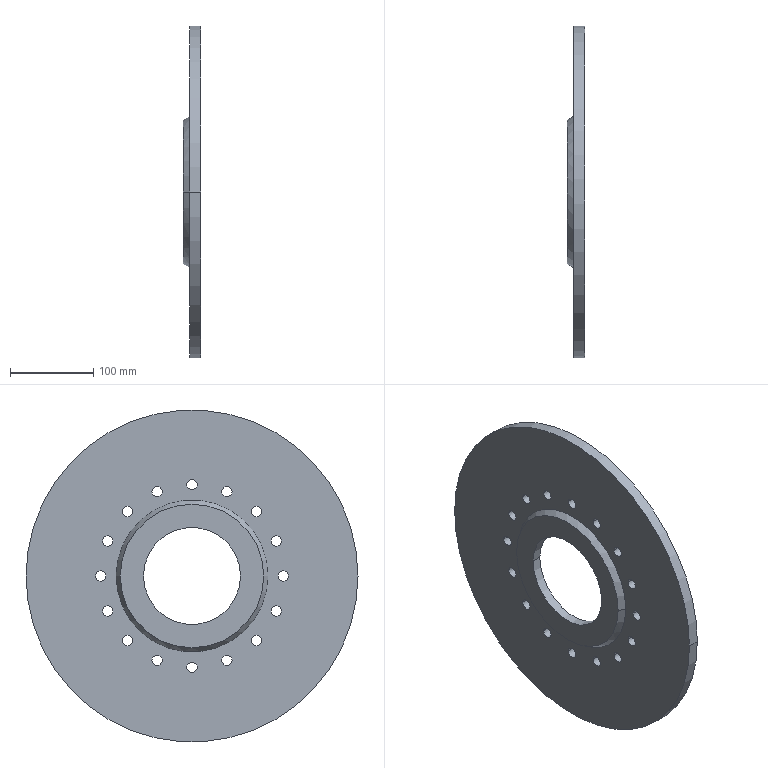Part | NX | features BREP 1 | 1 solid | 44 faces | box 21.5 x 400 x 400 mm | volume 1510380 mm3 | cylinder 38 | plane 4 | cone 2 | commonest cylinder face diameters 12.5 x32 117 x2 173 x2 400 x2
STEP:
#1=CARTESIAN_POINT('',(-403.355,-86.5,0.));
#2=VERTEX_POINT('',#1);
#3=CARTESIAN_POINT('',(-395.355,-91.5,0.));
#4=VERTEX_POINT('',#3);
#5=CARTESIAN_POINT('',(-403.355,-86.5,0.));
#6=DIRECTION('',(0.848,-0.53,0.));
#7=VECTOR('',#6,1000.);
#8=LINE('',#5,#7);
#9=EDGE_CURVE('',#2,#4,#8,.T.);
#10=ORIENTED_EDGE('',*,*,#9,.T.);
#11=CARTESIAN_POINT('',(-395.355,91.5,0.));
#12=VERTEX_POINT('',#11);
#13=CARTESIAN_POINT('',(-395.355,0.,0.));
#14=DIRECTION('',(-1.,0.,0.));
#15=DIRECTION('',(0.,-1.,0.));
#16=AXIS2_PLACEMENT_3D('',#13,#14,#15);
#17=CIRCLE('',#16,91.5);
#18=EDGE_CURVE('',#4,#12,#17,.T.);
#19=ORIENTED_EDGE('',*,*,#18,.T.);
#20=CARTESIAN_POINT('',(-403.355,86.5,0.));
#21=VERTEX_POINT('',#20);
#22=CARTESIAN_POINT('',(-403.355,86.5,0.));
#23=DIRECTION('',(0.848,0.53,0.));
#24=VECTOR('',#23,1000.);
#25=LINE('',#22,#24);
#26=EDGE_CURVE('',#21,#12,#25,.T.);
#27=ORIENTED_EDGE('',*,*,#26,.F.);
#28=CARTESIAN_POINT('',(-403.355,0.,0.));
#29=DIRECTION('',(-1.,0.,0.));
#30=DIRECTION('',(0.,-1.,0.));
#31=AXIS2_PLACEMENT_3D('',#28,#29,#30);
#32=CIRCLE('',#31,86.5);
#33=EDGE_CURVE('',#2,#21,#32,.T.);
#34=ORIENTED_EDGE('',*,*,#33,.F.);
#35=EDGE_LOOP('',(#10,#19,#27,#34));
#36=FACE_BOUND('',#35,.T.);
#37=CARTESIAN_POINT('',(-403.355,0.,0.));
#38=DIRECTION('',(1.,0.,0.));
#39=DIRECTION('',(0.,-1.,0.));
#40=AXIS2_PLACEMENT_3D('',#37,#38,#39);
#41=CONICAL_SURFACE('',#40,86.5,0.5586);
#42=ADVANCED_FACE('',(#36),#41,.T.);
#43=CARTESIAN_POINT('',(-395.355,107.877,42.095));
#44=VERTEX_POINT('',#43);
#45=CARTESIAN_POINT('',(-381.855,107.877,42.095));
#46=VERTEX_POINT('',#45);
#47=CARTESIAN_POINT('',(-381.855,107.877,42.095));
#48=DIRECTION('',(-1.,0.,0.));
#49=VECTOR('',#48,1000.);
#50=LINE('',#47,#49);
#51=EDGE_CURVE('',#44,#46,#50,.F.);
#52=ORIENTED_EDGE('',*,*,#51,.F.);
#53=CARTESIAN_POINT('',(-395.355,95.377,42.095));
#54=VERTEX_POINT('',#53);
#55=CARTESIAN_POINT('',(-395.355,101.627,42.095));
#56=DIRECTION('',(-1.,0.,0.));
#57=DIRECTION('',(0.,-1.,0.));
#58=AXIS2_PLACEMENT_3D('',#55,#56,#57);
#59=CIRCLE('',#58,6.25);
#60=EDGE_CURVE('',#44,#54,#59,.T.);
#61=ORIENTED_EDGE('',*,*,#60,.T.);
#62=CARTESIAN_POINT('',(-381.855,95.377,42.095));
#63=VERTEX_POINT('',#62);
#64=CARTESIAN_POINT('',(-381.855,95.377,42.095));
#65=DIRECTION('',(-1.,0.,0.));
#66=VECTOR('',#65,1000.);
#67=LINE('',#64,#66);
#68=EDGE_CURVE('',#54,#63,#67,.F.);
#69=ORIENTED_EDGE('',*,*,#68,.T.);
#70=CARTESIAN_POINT('',(-381.855,101.627,42.095));
#71=DIRECTION('',(-1.,0.,0.));
#72=DIRECTION('',(0.,-1.,0.));
#73=AXIS2_PLACEMENT_3D('',#70,#71,#72);
#74=CIRCLE('',#73,6.25);
#75=EDGE_CURVE('',#46,#63,#74,.T.);
#76=ORIENTED_EDGE('',*,*,#75,.F.);
#77=EDGE_LOOP('',(#52,#61,#69,#76));
#78=FACE_BOUND('',#77,.T.);
#79=CARTESIAN_POINT('',(-381.855,101.627,42.095));
#80=DIRECTION('',(-1.,0.,0.));
#81=DIRECTION('',(0.,1.,0.));
#82=AXIS2_PLACEMENT_3D('',#79,#80,#81);
#83=CYLINDRICAL_SURFACE('',#82,6.25);
#84=ADVANCED_FACE('',(#78),#83,.F.);
#85=CARTESIAN_POINT('',(-395.355,84.032,77.782));
#86=VERTEX_POINT('',#85);
#87=CARTESIAN_POINT('',(-381.855,84.032,77.782));
#88=VERTEX_POINT('',#87);
#89=CARTESIAN_POINT('',(-381.855,84.032,77.782));
#90=DIRECTION('',(-1.,0.,0.));
#91=VECTOR('',#90,1000.);
#92=LINE('',#89,#91);
#93=EDGE_CURVE('',#86,#88,#92,.F.);
#94=ORIENTED_EDGE('',*,*,#93,.F.);
#95=CARTESIAN_POINT('',(-395.355,71.532,77.782));
#96=VERTEX_POINT('',#95);
#97=CARTESIAN_POINT('',(-395.355,77.782,77.782));
#98=DIRECTION('',(-1.,0.,0.));
#99=DIRECTION('',(0.,-1.,0.));
#100=AXIS2_PLACEMENT_3D('',#97,#98,#99);
#101=CIRCLE('',#100,6.25);
#102=EDGE_CURVE('',#86,#96,#101,.T.);
#103=ORIENTED_EDGE('',*,*,#102,.T.);
#104=CARTESIAN_POINT('',(-381.855,71.532,77.782));
#105=VERTEX_POINT('',#104);
#106=CARTESIAN_POINT('',(-381.855,71.532,77.782));
#107=DIRECTION('',(-1.,0.,0.));
#108=VECTOR('',#107,1000.);
#109=LINE('',#106,#108);
#110=EDGE_CURVE('',#96,#105,#109,.F.);
#111=ORIENTED_EDGE('',*,*,#110,.T.);
#112=CARTESIAN_POINT('',(-381.855,77.782,77.782));
#113=DIRECTION('',(-1.,0.,0.));
#114=DIRECTION('',(0.,-1.,0.));
#115=AXIS2_PLACEMENT_3D('',#112,#113,#114);
#116=CIRCLE('',#115,6.25);
#117=EDGE_CURVE('',#88,#105,#116,.T.);
#118=ORIENTED_EDGE('',*,*,#117,.F.);
#119=EDGE_LOOP('',(#94,#103,#111,#118));
#120=FACE_BOUND('',#119,.T.);
#121=CARTESIAN_POINT('',(-381.855,77.782,77.782));
#122=DIRECTION('',(-1.,0.,0.));
#123=DIRECTION('',(0.,1.,0.));
#124=AXIS2_PLACEMENT_3D('',#121,#122,#123);
#125=CYLINDRICAL_SURFACE('',#124,6.25);
#126=ADVANCED_FACE('',(#120),#125,.F.);
#127=CARTESIAN_POINT('',(-395.355,48.345,101.627));
#128=VERTEX_POINT('',#127);
#129=CARTESIAN_POINT('',(-381.855,48.345,101.627));
#130=VERTEX_POINT('',#129);
#131=CARTESIAN_POINT('',(-381.855,48.345,101.627));
#132=DIRECTION('',(-1.,0.,0.));
#133=VECTOR('',#132,1000.);
#134=LINE('',#131,#133);
#135=EDGE_CURVE('',#128,#130,#134,.F.);
#136=ORIENTED_EDGE('',*,*,#135,.F.);
#137=CARTESIAN_POINT('',(-395.355,35.845,101.627));
#138=VERTEX_POINT('',#137);
#139=CARTESIAN_POINT('',(-395.355,42.095,101.627));
#140=DIRECTION('',(-1.,0.,0.));
#141=DIRECTION('',(0.,-1.,0.));
#142=AXIS2_PLACEMENT_3D('',#139,#140,#141);
#143=CIRCLE('',#142,6.25);
#144=EDGE_CURVE('',#128,#138,#143,.T.);
#145=ORIENTED_EDGE('',*,*,#144,.T.);
#146=CARTESIAN_POINT('',(-381.855,35.845,101.627));
#147=VERTEX_POINT('',#146);
#148=CARTESIAN_POINT('',(-381.855,35.845,101.627));
#149=DIRECTION('',(-1.,0.,0.));
#150=VECTOR('',#149,1000.);
#151=LINE('',#148,#150);
#152=EDGE_CURVE('',#138,#147,#151,.F.);
#153=ORIENTED_EDGE('',*,*,#152,.T.);
#154=CARTESIAN_POINT('',(-381.855,42.095,101.627));
#155=DIRECTION('',(-1.,0.,0.));
#156=DIRECTION('',(0.,-1.,0.));
#157=AXIS2_PLACEMENT_3D('',#154,#155,#156);
#158=CIRCLE('',#157,6.25);
#159=EDGE_CURVE('',#130,#147,#158,.T.);
#160=ORIENTED_EDGE('',*,*,#159,.F.);
#161=EDGE_LOOP('',(#136,#145,#153,#160));
#162=FACE_BOUND('',#161,.T.);
#163=CARTESIAN_POINT('',(-381.855,42.095,101.627));
#164=DIRECTION('',(-1.,0.,0.));
#165=DIRECTION('',(0.,1.,0.));
#166=AXIS2_PLACEMENT_3D('',#163,#164,#165);
#167=CYLINDRICAL_SURFACE('',#166,6.25);
#168=ADVANCED_FACE('',(#162),#167,.F.);
#169=CARTESIAN_POINT('',(-395.355,6.25,110.));
#170=VERTEX_POINT('',#169);
#171=CARTESIAN_POINT('',(-381.855,6.25,110.));
#172=VERTEX_POINT('',#171);
#173=CARTESIAN_POINT('',(-381.855,6.25,110.));
#174=DIRECTION('',(-1.,0.,0.));
#175=VECTOR('',#174,1000.);
#176=LINE('',#173,#175);
#177=EDGE_CURVE('',#170,#172,#176,.F.);
#178=ORIENTED_EDGE('',*,*,#177,.F.);
#179=CARTESIAN_POINT('',(-395.355,-6.25,110.));
#180=VERTEX_POINT('',#179);
#181=CARTESIAN_POINT('',(-395.355,0.,110.));
#182=DIRECTION('',(-1.,0.,0.));
#183=DIRECTION('',(0.,-1.,0.));
#184=AXIS2_PLACEMENT_3D('',#181,#182,#183);
#185=CIRCLE('',#184,6.25);
#186=EDGE_CURVE('',#170,#180,#185,.T.);
#187=ORIENTED_EDGE('',*,*,#186,.T.);
#188=CARTESIAN_POINT('',(-381.855,-6.25,110.));
#189=VERTEX_POINT('',#188);
#190=CARTESIAN_POINT('',(-381.855,-6.25,110.));
#191=DIRECTION('',(-1.,0.,0.));
#192=VECTOR('',#191,1000.);
#193=LINE('',#190,#192);
#194=EDGE_CURVE('',#180,#189,#193,.F.);
#195=ORIENTED_EDGE('',*,*,#194,.T.);
#196=CARTESIAN_POINT('',(-381.855,0.,110.));
#197=DIRECTION('',(-1.,0.,0.));
#198=DIRECTION('',(0.,-1.,0.));
#199=AXIS2_PLACEMENT_3D('',#196,#197,#198);
#200=CIRCLE('',#199,6.25);
#201=EDGE_CURVE('',#172,#189,#200,.T.);
#202=ORIENTED_EDGE('',*,*,#201,.F.);
#203=EDGE_LOOP('',(#178,#187,#195,#202));
#204=FACE_BOUND('',#203,.T.);
#205=CARTESIAN_POINT('',(-381.855,0.,110.));
#206=DIRECTION('',(-1.,0.,0.));
#207=DIRECTION('',(0.,1.,0.));
#208=AXIS2_PLACEMENT_3D('',#205,#206,#207);
#209=CYLINDRICAL_SURFACE('',#208,6.25);
#210=ADVANCED_FACE('',(#204),#209,.F.);
#211=CARTESIAN_POINT('',(-395.355,-35.845,101.627));
#212=VERTEX_POINT('',#211);
#213=CARTESIAN_POINT('',(-381.855,-35.845,101.627));
#214=VERTEX_POINT('',#213);
#215=CARTESIAN_POINT('',(-381.855,-35.845,101.627));
#216=DIRECTION('',(-1.,0.,0.));
#217=VECTOR('',#216,1000.);
#218=LINE('',#215,#217);
#219=EDGE_CURVE('',#212,#214,#218,.F.);
#220=ORIENTED_EDGE('',*,*,#219,.F.);
#221=CARTESIAN_POINT('',(-395.355,-48.345,101.627));
#222=VERTEX_POINT('',#221);
#223=CARTESIAN_POINT('',(-395.355,-42.095,101.627));
#224=DIRECTION('',(-1.,0.,0.));
#225=DIRECTION('',(0.,-1.,0.));
#226=AXIS2_PLACEMENT_3D('',#223,#224,#225);
#227=CIRCLE('',#226,6.25);
#228=EDGE_CURVE('',#212,#222,#227,.T.);
#229=ORIENTED_EDGE('',*,*,#228,.T.);
#230=CARTESIAN_POINT('',(-381.855,-48.345,101.627));
#231=VERTEX_POINT('',#230);
#232=CARTESIAN_POINT('',(-381.855,-48.345,101.627));
#233=DIRECTION('',(-1.,0.,0.));
#234=VECTOR('',#233,1000.);
#235=LINE('',#232,#234);
#236=EDGE_CURVE('',#222,#231,#235,.F.);
#237=ORIENTED_EDGE('',*,*,#236,.T.);
#238=CARTESIAN_POINT('',(-381.855,-42.095,101.627));
#239=DIRECTION('',(-1.,0.,0.));
#240=DIRECTION('',(0.,-1.,0.));
#241=AXIS2_PLACEMENT_3D('',#238,#239,#240);
#242=CIRCLE('',#241,6.25);
#243=EDGE_CURVE('',#214,#231,#242,.T.);
#244=ORIENTED_EDGE('',*,*,#243,.F.);
#245=EDGE_LOOP('',(#220,#229,#237,#244));
#246=FACE_BOUND('',#245,.T.);
#247=CARTESIAN_POINT('',(-381.855,-42.095,101.627));
#248=DIRECTION('',(-1.,0.,0.));
#249=DIRECTION('',(0.,1.,0.));
#250=AXIS2_PLACEMENT_3D('',#247,#248,#249);
#251=CYLINDRICAL_SURFACE('',#250,6.25);
#252=ADVANCED_FACE('',(#246),#251,.F.);
#253=CARTESIAN_POINT('',(-395.355,-71.532,77.782));
#254=VERTEX_POINT('',#253);
#255=CARTESIAN_POINT('',(-381.855,-71.532,77.782));
#256=VERTEX_POINT('',#255);
#257=CARTESIAN_POINT('',(-381.855,-71.532,77.782));
#258=DIRECTION('',(-1.,0.,0.));
#259=VECTOR('',#258,1000.);
#260=LINE('',#257,#259);
#261=EDGE_CURVE('',#254,#256,#260,.F.);
#262=ORIENTED_EDGE('',*,*,#261,.F.);
#263=CARTESIAN_POINT('',(-395.355,-84.032,77.782));
#264=VERTEX_POINT('',#263);
#265=CARTESIAN_POINT('',(-395.355,-77.782,77.782));
#266=DIRECTION('',(-1.,0.,0.));
#267=DIRECTION('',(0.,-1.,0.));
#268=AXIS2_PLACEMENT_3D('',#265,#266,#267);
#269=CIRCLE('',#268,6.25);
#270=EDGE_CURVE('',#254,#264,#269,.T.);
#271=ORIENTED_EDGE('',*,*,#270,.T.);
#272=CARTESIAN_POINT('',(-381.855,-84.032,77.782));
#273=VERTEX_POINT('',#272);
#274=CARTESIAN_POINT('',(-381.855,-84.032,77.782));
#275=DIRECTION('',(-1.,0.,0.));
#276=VECTOR('',#275,1000.);
#277=LINE('',#274,#276);
#278=EDGE_CURVE('',#264,#273,#277,.F.);
#279=ORIENTED_EDGE('',*,*,#278,.T.);
#280=CARTESIAN_POINT('',(-381.855,-77.782,77.782));
#281=DIRECTION('',(-1.,0.,0.));
#282=DIRECTION('',(0.,-1.,0.));
#283=AXIS2_PLACEMENT_3D('',#280,#281,#282);
#284=CIRCLE('',#283,6.25);
#285=EDGE_CURVE('',#256,#273,#284,.T.);
#286=ORIENTED_EDGE('',*,*,#285,.F.);
#287=EDGE_LOOP('',(#262,#271,#279,#286));
#288=FACE_BOUND('',#287,.T.);
#289=CARTESIAN_POINT('',(-381.855,-77.782,77.782));
#290=DIRECTION('',(-1.,0.,0.));
#291=DIRECTION('',(0.,1.,0.));
#292=AXIS2_PLACEMENT_3D('',#289,#290,#291);
#293=CYLINDRICAL_SURFACE('',#292,6.25);
#294=ADVANCED_FACE('',(#288),#293,.F.);
#295=CARTESIAN_POINT('',(-395.355,-95.377,42.095));
#296=VERTEX_POINT('',#295);
#297=CARTESIAN_POINT('',(-381.855,-95.377,42.095));
#298=VERTEX_POINT('',#297);
#299=CARTESIAN_POINT('',(-381.855,-95.377,42.095));
#300=DIRECTION('',(-1.,0.,0.));
#301=VECTOR('',#300,1000.);
#302=LINE('',#299,#301);
#303=EDGE_CURVE('',#296,#298,#302,.F.);
#304=ORIENTED_EDGE('',*,*,#303,.F.);
#305=CARTESIAN_POINT('',(-395.355,-107.877,42.095));
#306=VERTEX_POINT('',#305);
#307=CARTESIAN_POINT('',(-395.355,-101.627,42.095));
#308=DIRECTION('',(-1.,0.,0.));
#309=DIRECTION('',(0.,-1.,0.));
#310=AXIS2_PLACEMENT_3D('',#307,#308,#309);
#311=CIRCLE('',#310,6.25);
#312=EDGE_CURVE('',#296,#306,#311,.T.);
#313=ORIENTED_EDGE('',*,*,#312,.T.);
#314=CARTESIAN_POINT('',(-381.855,-107.877,42.095));
#315=VERTEX_POINT('',#314);
#316=CARTESIAN_POINT('',(-381.855,-107.877,42.095));
#317=DIRECTION('',(-1.,0.,0.));
#318=VECTOR('',#317,1000.);
#319=LINE('',#316,#318);
#320=EDGE_CURVE('',#306,#315,#319,.F.);
#321=ORIENTED_EDGE('',*,*,#320,.T.);
#322=CARTESIAN_POINT('',(-381.855,-101.627,42.095));
#323=DIRECTION('',(-1.,0.,0.));
#324=DIRECTION('',(0.,-1.,0.));
#325=AXIS2_PLACEMENT_3D('',#322,#323,#324);
#326=CIRCLE('',#325,6.25);
#327=EDGE_CURVE('',#298,#315,#326,.T.);
#328=ORIENTED_EDGE('',*,*,#327,.F.);
#329=EDGE_LOOP('',(#304,#313,#321,#328));
#330=FACE_BOUND('',#329,.T.);
#331=CARTESIAN_POINT('',(-381.855,-101.627,42.095));
#332=DIRECTION('',(-1.,0.,0.));
#333=DIRECTION('',(0.,1.,0.));
#334=AXIS2_PLACEMENT_3D('',#331,#332,#333);
#335=CYLINDRICAL_SURFACE('',#334,6.25);
#336=ADVANCED_FACE('',(#330),#335,.F.);
#337=CARTESIAN_POINT('',(-395.355,-103.75,0.));
#338=VERTEX_POINT('',#337);
#339=CARTESIAN_POINT('',(-381.855,-103.75,0.));
#340=VERTEX_POINT('',#339);
#341=CARTESIAN_POINT('',(-381.855,-103.75,0.));
#342=DIRECTION('',(-1.,0.,0.));
#343=VECTOR('',#342,1000.);
#344=LINE('',#341,#343);
#345=EDGE_CURVE('',#338,#340,#344,.F.);
#346=ORIENTED_EDGE('',*,*,#345,.F.);
#347=CARTESIAN_POINT('',(-395.355,-116.25,0.));
#348=VERTEX_POINT('',#347);
#349=CARTESIAN_POINT('',(-395.355,-110.,0.));
#350=DIRECTION('',(-1.,0.,0.));
#351=DIRECTION('',(0.,-1.,0.));
#352=AXIS2_PLACEMENT_3D('',#349,#350,#351);
#353=CIRCLE('',#352,6.25);
#354=EDGE_CURVE('',#338,#348,#353,.T.);
#355=ORIENTED_EDGE('',*,*,#354,.T.);
#356=CARTESIAN_POINT('',(-381.855,-116.25,0.));
#357=VERTEX_POINT('',#356);
#358=CARTESIAN_POINT('',(-381.855,-116.25,0.));
#359=DIRECTION('',(-1.,0.,0.));
#360=VECTOR('',#359,1000.);
#361=LINE('',#358,#360);
#362=EDGE_CURVE('',#348,#357,#361,.F.);
#363=ORIENTED_EDGE('',*,*,#362,.T.);
#364=CARTESIAN_POINT('',(-381.855,-110.,0.));
#365=DIRECTION('',(-1.,0.,0.));
#366=DIRECTION('',(0.,-1.,0.));
#367=AXIS2_PLACEMENT_3D('',#364,#365,#366);
#368=CIRCLE('',#367,6.25);
#369=EDGE_CURVE('',#340,#357,#368,.T.);
#370=ORIENTED_EDGE('',*,*,#369,.F.);
#371=EDGE_LOOP('',(#346,#355,#363,#370));
#372=FACE_BOUND('',#371,.T.);
#373=CARTESIAN_POINT('',(-381.855,-110.,0.));
#374=DIRECTION('',(-1.,0.,0.));
#375=DIRECTION('',(0.,1.,0.));
#376=AXIS2_PLACEMENT_3D('',#373,#374,#375);
#377=CYLINDRICAL_SURFACE('',#376,6.25);
#378=ADVANCED_FACE('',(#372),#377,.F.);
#379=CARTESIAN_POINT('',(-395.355,-95.377,-42.095));
#380=VERTEX_POINT('',#379);
#381=CARTESIAN_POINT('',(-381.855,-95.377,-42.095));
#382=VERTEX_POINT('',#381);
#383=CARTESIAN_POINT('',(-381.855,-95.377,-42.095));
#384=DIRECTION('',(-1.,0.,0.));
#385=VECTOR('',#384,1000.);
#386=LINE('',#383,#385);
#387=EDGE_CURVE('',#380,#382,#386,.F.);
#388=ORIENTED_EDGE('',*,*,#387,.F.);
#389=CARTESIAN_POINT('',(-395.355,-107.877,-42.095));
#390=VERTEX_POINT('',#389);
#391=CARTESIAN_POINT('',(-395.355,-101.627,-42.095));
#392=DIRECTION('',(-1.,0.,0.));
#393=DIRECTION('',(0.,-1.,0.));
#394=AXIS2_PLACEMENT_3D('',#391,#392,#393);
#395=CIRCLE('',#394,6.25);
#396=EDGE_CURVE('',#380,#390,#395,.T.);
#397=ORIENTED_EDGE('',*,*,#396,.T.);
#398=CARTESIAN_POINT('',(-381.855,-107.877,-42.095));
#399=VERTEX_POINT('',#398);
#400=CARTESIAN_POINT('',(-381.855,-107.877,-42.095));
#401=DIRECTION('',(-1.,0.,0.));
#402=VECTOR('',#401,1000.);
#403=LINE('',#400,#402);
#404=EDGE_CURVE('',#390,#399,#403,.F.);
#405=ORIENTED_EDGE('',*,*,#404,.T.);
#406=CARTESIAN_POINT('',(-381.855,-101.627,-42.095));
#407=DIRECTION('',(-1.,0.,0.));
#408=DIRECTION('',(0.,-1.,0.));
#409=AXIS2_PLACEMENT_3D('',#406,#407,#408);
#410=CIRCLE('',#409,6.25);
#411=EDGE_CURVE('',#382,#399,#410,.T.);
#412=ORIENTED_EDGE('',*,*,#411,.F.);
#413=EDGE_LOOP('',(#388,#397,#405,#412));
#414=FACE_BOUND('',#413,.T.);
#415=CARTESIAN_POINT('',(-381.855,-101.627,-42.095));
#416=DIRECTION('',(-1.,0.,0.));
#417=DIRECTION('',(0.,1.,0.));
#418=AXIS2_PLACEMENT_3D('',#415,#416,#417);
#419=CYLINDRICAL_SURFACE('',#418,6.25);
#420=ADVANCED_FACE('',(#414),#419,.F.);
#421=CARTESIAN_POINT('',(-395.355,-71.532,-77.782));
#422=VERTEX_POINT('',#421);
#423=CARTESIAN_POINT('',(-381.855,-71.532,-77.782));
#424=VERTEX_POINT('',#423);
#425=CARTESIAN_POINT('',(-381.855,-71.532,-77.782));
#426=DIRECTION('',(-1.,0.,0.));
#427=VECTOR('',#426,1000.);
#428=LINE('',#425,#427);
#429=EDGE_CURVE('',#422,#424,#428,.F.);
#430=ORIENTED_EDGE('',*,*,#429,.F.);
#431=CARTESIAN_POINT('',(-395.355,-84.032,-77.782));
#432=VERTEX_POINT('',#431);
#433=CARTESIAN_POINT('',(-395.355,-77.782,-77.782));
#434=DIRECTION('',(-1.,0.,0.));
#435=DIRECTION('',(0.,-1.,0.));
#436=AXIS2_PLACEMENT_3D('',#433,#434,#435);
#437=CIRCLE('',#436,6.25);
#438=EDGE_CURVE('',#422,#432,#437,.T.);
#439=ORIENTED_EDGE('',*,*,#438,.T.);
#440=CARTESIAN_POINT('',(-381.855,-84.032,-77.782));
#441=VERTEX_POINT('',#440);
#442=CARTESIAN_POINT('',(-381.855,-84.032,-77.782));
#443=DIRECTION('',(-1.,0.,0.));
#444=VECTOR('',#443,1000.);
#445=LINE('',#442,#444);
#446=EDGE_CURVE('',#432,#441,#445,.F.);
#447=ORIENTED_EDGE('',*,*,#446,.T.);
#448=CARTESIAN_POINT('',(-381.855,-77.782,-77.782));
#449=DIRECTION('',(-1.,0.,0.));
#450=DIRECTION('',(0.,-1.,0.));
#451=AXIS2_PLACEMENT_3D('',#448,#449,#450);
#452=CIRCLE('',#451,6.25);
#453=EDGE_CURVE('',#424,#441,#452,.T.);
#454=ORIENTED_EDGE('',*,*,#453,.F.);
#455=EDGE_LOOP('',(#430,#439,#447,#454));
#456=FACE_BOUND('',#455,.T.);
#457=CARTESIAN_POINT('',(-381.855,-77.782,-77.782));
#458=DIRECTION('',(-1.,0.,0.));
#459=DIRECTION('',(0.,1.,0.));
#460=AXIS2_PLACEMENT_3D('',#457,#458,#459);
#461=CYLINDRICAL_SURFACE('',#460,6.25);
#462=ADVANCED_FACE('',(#456),#461,.F.);
#463=CARTESIAN_POINT('',(-395.355,-35.845,-101.627));
#464=VERTEX_POINT('',#463);
#465=CARTESIAN_POINT('',(-381.855,-35.845,-101.627));
#466=VERTEX_POINT('',#465);
#467=CARTESIAN_POINT('',(-381.855,-35.845,-101.627));
#468=DIRECTION('',(-1.,0.,0.));
#469=VECTOR('',#468,1000.);
#470=LINE('',#467,#469);
#471=EDGE_CURVE('',#464,#466,#470,.F.);
#472=ORIENTED_EDGE('',*,*,#471,.F.);
#473=CARTESIAN_POINT('',(-395.355,-48.345,-101.627));
#474=VERTEX_POINT('',#473);
#475=CARTESIAN_POINT('',(-395.355,-42.095,-101.627));
#476=DIRECTION('',(-1.,0.,0.));
#477=DIRECTION('',(0.,-1.,0.));
#478=AXIS2_PLACEMENT_3D('',#475,#476,#477);
#479=CIRCLE('',#478,6.25);
#480=EDGE_CURVE('',#464,#474,#479,.T.);
#481=ORIENTED_EDGE('',*,*,#480,.T.);
#482=CARTESIAN_POINT('',(-381.855,-48.345,-101.627));
#483=VERTEX_POINT('',#482);
#484=CARTESIAN_POINT('',(-381.855,-48.345,-101.627));
#485=DIRECTION('',(-1.,0.,0.));
#486=VECTOR('',#485,1000.);
#487=LINE('',#484,#486);
#488=EDGE_CURVE('',#474,#483,#487,.F.);
#489=ORIENTED_EDGE('',*,*,#488,.T.);
#490=CARTESIAN_POINT('',(-381.855,-42.095,-101.627));
#491=DIRECTION('',(-1.,0.,0.));
#492=DIRECTION('',(0.,-1.,0.));
#493=AXIS2_PLACEMENT_3D('',#490,#491,#492);
#494=CIRCLE('',#493,6.25);
#495=EDGE_CURVE('',#466,#483,#494,.T.);
#496=ORIENTED_EDGE('',*,*,#495,.F.);
#497=EDGE_LOOP('',(#472,#481,#489,#496));
#498=FACE_BOUND('',#497,.T.);
#499=CARTESIAN_POINT('',(-381.855,-42.095,-101.627));
#500=DIRECTION('',(-1.,0.,0.));
#501=DIRECTION('',(0.,1.,0.));
#502=AXIS2_PLACEMENT_3D('',#499,#500,#501);
#503=CYLINDRICAL_SURFACE('',#502,6.25);
#504=ADVANCED_FACE('',(#498),#503,.F.);
#505=CARTESIAN_POINT('',(-395.355,6.25,-110.));
#506=VERTEX_POINT('',#505);
#507=CARTESIAN_POINT('',(-381.855,6.25,-110.));
#508=VERTEX_POINT('',#507);
#509=CARTESIAN_POINT('',(-381.855,6.25,-110.));
#510=DIRECTION('',(-1.,0.,0.));
#511=VECTOR('',#510,1000.);
#512=LINE('',#509,#511);
#513=EDGE_CURVE('',#506,#508,#512,.F.);
#514=ORIENTED_EDGE('',*,*,#513,.F.);
#515=CARTESIAN_POINT('',(-395.355,-6.25,-110.));
#516=VERTEX_POINT('',#515);
#517=CARTESIAN_POINT('',(-395.355,0.,-110.));
#518=DIRECTION('',(-1.,0.,0.));
#519=DIRECTION('',(0.,-1.,0.));
#520=AXIS2_PLACEMENT_3D('',#517,#518,#519);
#521=CIRCLE('',#520,6.25);
#522=EDGE_CURVE('',#506,#516,#521,.T.);
#523=ORIENTED_EDGE('',*,*,#522,.T.);
#524=CARTESIAN_POINT('',(-381.855,-6.25,-110.));
#525=VERTEX_POINT('',#524);
#526=CARTESIAN_POINT('',(-381.855,-6.25,-110.));
#527=DIRECTION('',(-1.,0.,0.));
#528=VECTOR('',#527,1000.);
#529=LINE('',#526,#528);
#530=EDGE_CURVE('',#516,#525,#529,.F.);
#531=ORIENTED_EDGE('',*,*,#530,.T.);
#532=CARTESIAN_POINT('',(-381.855,0.,-110.));
#533=DIRECTION('',(-1.,0.,0.));
#534=DIRECTION('',(0.,-1.,0.));
#535=AXIS2_PLACEMENT_3D('',#532,#533,#534);
#536=CIRCLE('',#535,6.25);
#537=EDGE_CURVE('',#508,#525,#536,.T.);
#538=ORIENTED_EDGE('',*,*,#537,.F.);
#539=EDGE_LOOP('',(#514,#523,#531,#538));
#540=FACE_BOUND('',#539,.T.);
#541=CARTESIAN_POINT('',(-381.855,0.,-110.));
#542=DIRECTION('',(-1.,0.,0.));
#543=DIRECTION('',(0.,1.,0.));
#544=AXIS2_PLACEMENT_3D('',#541,#542,#543);
#545=CYLINDRICAL_SURFACE('',#544,6.25);
#546=ADVANCED_FACE('',(#540),#545,.F.);
#547=CARTESIAN_POINT('',(-395.355,48.345,-101.627));
#548=VERTEX_POINT('',#547);
#549=CARTESIAN_POINT('',(-381.855,48.345,-101.627));
#550=VERTEX_POINT('',#549);
#551=CARTESIAN_POINT('',(-381.855,48.345,-101.627));
#552=DIRECTION('',(-1.,0.,0.));
#553=VECTOR('',#552,1000.);
#554=LINE('',#551,#553);
#555=EDGE_CURVE('',#548,#550,#554,.F.);
#556=ORIENTED_EDGE('',*,*,#555,.F.);
#557=CARTESIAN_POINT('',(-395.355,35.845,-101.627));
#558=VERTEX_POINT('',#557);
#559=CARTESIAN_POINT('',(-395.355,42.095,-101.627));
#560=DIRECTION('',(-1.,0.,0.));
#561=DIRECTION('',(0.,-1.,0.));
#562=AXIS2_PLACEMENT_3D('',#559,#560,#561);
#563=CIRCLE('',#562,6.25);
#564=EDGE_CURVE('',#548,#558,#563,.T.);
#565=ORIENTED_EDGE('',*,*,#564,.T.);
#566=CARTESIAN_POINT('',(-381.855,35.845,-101.627));
#567=VERTEX_POINT('',#566);
#568=CARTESIAN_POINT('',(-381.855,35.845,-101.627));
#569=DIRECTION('',(-1.,0.,0.));
#570=VECTOR('',#569,1000.);
#571=LINE('',#568,#570);
#572=EDGE_CURVE('',#558,#567,#571,.F.);
#573=ORIENTED_EDGE('',*,*,#572,.T.);
#574=CARTESIAN_POINT('',(-381.855,42.095,-101.627));
#575=DIRECTION('',(-1.,0.,0.));
#576=DIRECTION('',(0.,-1.,0.));
#577=AXIS2_PLACEMENT_3D('',#574,#575,#576);
#578=CIRCLE('',#577,6.25);
#579=EDGE_CURVE('',#550,#567,#578,.T.);
#580=ORIENTED_EDGE('',*,*,#579,.F.);
#581=EDGE_LOOP('',(#556,#565,#573,#580));
#582=FACE_BOUND('',#581,.T.);
#583=CARTESIAN_POINT('',(-381.855,42.095,-101.627));
#584=DIRECTION('',(-1.,0.,0.));
#585=DIRECTION('',(0.,1.,0.));
#586=AXIS2_PLACEMENT_3D('',#583,#584,#585);
#587=CYLINDRICAL_SURFACE('',#586,6.25);
#588=ADVANCED_FACE('',(#582),#587,.F.);
#589=CARTESIAN_POINT('',(-395.355,84.032,-77.782));
#590=VERTEX_POINT('',#589);
#591=CARTESIAN_POINT('',(-381.855,84.032,-77.782));
#592=VERTEX_POINT('',#591);
#593=CARTESIAN_POINT('',(-381.855,84.032,-77.782));
#594=DIRECTION('',(-1.,0.,0.));
#595=VECTOR('',#594,1000.);
#596=LINE('',#593,#595);
#597=EDGE_CURVE('',#590,#592,#596,.F.);
#598=ORIENTED_EDGE('',*,*,#597,.F.);
#599=CARTESIAN_POINT('',(-395.355,71.532,-77.782));
#600=VERTEX_POINT('',#599);
#601=CARTESIAN_POINT('',(-395.355,77.782,-77.782));
#602=DIRECTION('',(-1.,0.,0.));
#603=DIRECTION('',(0.,-1.,0.));
#604=AXIS2_PLACEMENT_3D('',#601,#602,#603);
#605=CIRCLE('',#604,6.25);
#606=EDGE_CURVE('',#590,#600,#605,.T.);
#607=ORIENTED_EDGE('',*,*,#606,.T.);
#608=CARTESIAN_POINT('',(-381.855,71.532,-77.782));
#609=VERTEX_POINT('',#608);
#610=CARTESIAN_POINT('',(-381.855,71.532,-77.782));
#611=DIRECTION('',(-1.,0.,0.));
#612=VECTOR('',#611,1000.);
#613=LINE('',#610,#612);
#614=EDGE_CURVE('',#600,#609,#613,.F.);
#615=ORIENTED_EDGE('',*,*,#614,.T.);
#616=CARTESIAN_POINT('',(-381.855,77.782,-77.782));
#617=DIRECTION('',(-1.,0.,0.));
#618=DIRECTION('',(0.,-1.,0.));
#619=AXIS2_PLACEMENT_3D('',#616,#617,#618);
#620=CIRCLE('',#619,6.25);
#621=EDGE_CURVE('',#592,#609,#620,.T.);
#622=ORIENTED_EDGE('',*,*,#621,.F.);
#623=EDGE_LOOP('',(#598,#607,#615,#622));
#624=FACE_BOUND('',#623,.T.);
#625=CARTESIAN_POINT('',(-381.855,77.782,-77.782));
#626=DIRECTION('',(-1.,0.,0.));
#627=DIRECTION('',(0.,1.,0.));
#628=AXIS2_PLACEMENT_3D('',#625,#626,#627);
#629=CYLINDRICAL_SURFACE('',#628,6.25);
#630=ADVANCED_FACE('',(#624),#629,.F.);
#631=CARTESIAN_POINT('',(-395.355,107.877,-42.095));
#632=VERTEX_POINT('',#631);
#633=CARTESIAN_POINT('',(-381.855,107.877,-42.095));
#634=VERTEX_POINT('',#633);
#635=CARTESIAN_POINT('',(-381.855,107.877,-42.095));
#636=DIRECTION('',(-1.,0.,0.));
#637=VECTOR('',#636,1000.);
#638=LINE('',#635,#637);
#639=EDGE_CURVE('',#632,#634,#638,.F.);
#640=ORIENTED_EDGE('',*,*,#639,.F.);
#641=CARTESIAN_POINT('',(-395.355,95.377,-42.095));
#642=VERTEX_POINT('',#641);
#643=CARTESIAN_POINT('',(-395.355,101.627,-42.095));
#644=DIRECTION('',(-1.,0.,0.));
#645=DIRECTION('',(0.,-1.,0.));
#646=AXIS2_PLACEMENT_3D('',#643,#644,#645);
#647=CIRCLE('',#646,6.25);
#648=EDGE_CURVE('',#632,#642,#647,.T.);
#649=ORIENTED_EDGE('',*,*,#648,.T.);
#650=CARTESIAN_POINT('',(-381.855,95.377,-42.095));
#651=VERTEX_POINT('',#650);
#652=CARTESIAN_POINT('',(-381.855,95.377,-42.095));
#653=DIRECTION('',(-1.,0.,0.));
#654=VECTOR('',#653,1000.);
#655=LINE('',#652,#654);
#656=EDGE_CURVE('',#642,#651,#655,.F.);
#657=ORIENTED_EDGE('',*,*,#656,.T.);
#658=CARTESIAN_POINT('',(-381.855,101.627,-42.095));
#659=DIRECTION('',(-1.,0.,0.));
#660=DIRECTION('',(0.,-1.,0.));
#661=AXIS2_PLACEMENT_3D('',#658,#659,#660);
#662=CIRCLE('',#661,6.25);
#663=EDGE_CURVE('',#634,#651,#662,.T.);
#664=ORIENTED_EDGE('',*,*,#663,.F.);
#665=EDGE_LOOP('',(#640,#649,#657,#664));
#666=FACE_BOUND('',#665,.T.);
#667=CARTESIAN_POINT('',(-381.855,101.627,-42.095));
#668=DIRECTION('',(-1.,0.,0.));
#669=DIRECTION('',(0.,1.,0.));
#670=AXIS2_PLACEMENT_3D('',#667,#668,#669);
#671=CYLINDRICAL_SURFACE('',#670,6.25);
#672=ADVANCED_FACE('',(#666),#671,.F.);
#673=CARTESIAN_POINT('',(-395.355,116.25,0.));
#674=VERTEX_POINT('',#673);
#675=CARTESIAN_POINT('',(-381.855,116.25,0.));
#676=VERTEX_POINT('',#675);
#677=CARTESIAN_POINT('',(-381.855,116.25,0.));
#678=DIRECTION('',(-1.,0.,0.));
#679=VECTOR('',#678,1000.);
#680=LINE('',#677,#679);
#681=EDGE_CURVE('',#674,#676,#680,.F.);
#682=ORIENTED_EDGE('',*,*,#681,.F.);
#683=CARTESIAN_POINT('',(-395.355,103.75,0.));
#684=VERTEX_POINT('',#683);
#685=CARTESIAN_POINT('',(-395.355,110.,0.));
#686=DIRECTION('',(-1.,0.,0.));
#687=DIRECTION('',(0.,-1.,0.));
#688=AXIS2_PLACEMENT_3D('',#685,#686,#687);
#689=CIRCLE('',#688,6.25);
#690=EDGE_CURVE('',#674,#684,#689,.T.);
#691=ORIENTED_EDGE('',*,*,#690,.T.);
#692=CARTESIAN_POINT('',(-381.855,103.75,0.));
#693=VERTEX_POINT('',#692);
#694=CARTESIAN_POINT('',(-381.855,103.75,0.));
#695=DIRECTION('',(-1.,0.,0.));
#696=VECTOR('',#695,1000.);
#697=LINE('',#694,#696);
#698=EDGE_CURVE('',#684,#693,#697,.F.);
#699=ORIENTED_EDGE('',*,*,#698,.T.);
#700=CARTESIAN_POINT('',(-381.855,110.,0.));
#701=DIRECTION('',(-1.,0.,0.));
#702=DIRECTION('',(0.,-1.,0.));
#703=AXIS2_PLACEMENT_3D('',#700,#701,#702);
#704=CIRCLE('',#703,6.25);
#705=EDGE_CURVE('',#676,#693,#704,.T.);
#706=ORIENTED_EDGE('',*,*,#705,.F.);
#707=EDGE_LOOP('',(#682,#691,#699,#706));
#708=FACE_BOUND('',#707,.T.);
#709=CARTESIAN_POINT('',(-381.855,110.,0.));
#710=DIRECTION('',(-1.,0.,0.));
#711=DIRECTION('',(0.,1.,0.));
#712=AXIS2_PLACEMENT_3D('',#709,#710,#711);
#713=CYLINDRICAL_SURFACE('',#712,6.25);
#714=ADVANCED_FACE('',(#708),#713,.F.);
#715=CARTESIAN_POINT('',(-391.855,58.5,0.));
#716=VERTEX_POINT('',#715);
#717=CARTESIAN_POINT('',(-391.855,-58.5,0.));
#718=VERTEX_POINT('',#717);
#719=CARTESIAN_POINT('',(-391.855,0.,0.));
#720=DIRECTION('',(1.,0.,0.));
#721=DIRECTION('',(0.,1.,0.));
#722=AXIS2_PLACEMENT_3D('',#719,#720,#721);
#723=CIRCLE('',#722,58.5);
#724=EDGE_CURVE('',#716,#718,#723,.T.);
#725=ORIENTED_EDGE('',*,*,#724,.F.);
#726=CARTESIAN_POINT('',(-391.855,0.,0.));
#727=DIRECTION('',(1.,0.,0.));
#728=DIRECTION('',(0.,1.,0.));
#729=AXIS2_PLACEMENT_3D('',#726,#727,#728);
#730=CIRCLE('',#729,58.5);
#731=EDGE_CURVE('',#718,#716,#730,.T.);
#732=ORIENTED_EDGE('',*,*,#731,.F.);
#733=EDGE_LOOP('',(#725,#732));
#734=FACE_BOUND('',#733,.T.);
#735=CARTESIAN_POINT('',(-391.855,-86.5,0.));
#736=VERTEX_POINT('',#735);
#737=CARTESIAN_POINT('',(-391.855,86.5,0.));
#738=VERTEX_POINT('',#737);
#739=CARTESIAN_POINT('',(-391.855,0.,0.));
#740=DIRECTION('',(1.,0.,0.));
#741=DIRECTION('',(0.,1.,0.));
#742=AXIS2_PLACEMENT_3D('',#739,#740,#741);
#743=CIRCLE('',#742,86.5);
#744=EDGE_CURVE('',#736,#738,#743,.T.);
#745=ORIENTED_EDGE('',*,*,#744,.T.);
#746=CARTESIAN_POINT('',(-391.855,0.,0.));
#747=DIRECTION('',(1.,0.,0.));
#748=DIRECTION('',(0.,1.,0.));
#749=AXIS2_PLACEMENT_3D('',#746,#747,#748);
#750=CIRCLE('',#749,86.5);
#751=EDGE_CURVE('',#738,#736,#750,.T.);
#752=ORIENTED_EDGE('',*,*,#751,.T.);
#753=EDGE_LOOP('',(#745,#752));
#754=FACE_BOUND('',#753,.T.);
#755=CARTESIAN_POINT('',(-391.855,0.,0.));
#756=DIRECTION('',(1.,0.,0.));
#757=DIRECTION('',(0.,-1.,0.));
#758=AXIS2_PLACEMENT_3D('',#755,#756,#757);
#759=PLANE('',#758);
#760=ADVANCED_FACE('',(#734,#754),#759,.T.);
#761=CARTESIAN_POINT('',(-403.355,58.5,0.));
#762=VERTEX_POINT('',#761);
#763=CARTESIAN_POINT('',(-395.355,58.5,0.));
#764=DIRECTION('',(-1.,0.,0.));
#765=VECTOR('',#764,1000.);
#766=LINE('',#763,#765);
#767=EDGE_CURVE('',#762,#716,#766,.F.);
#768=ORIENTED_EDGE('',*,*,#767,.F.);
#769=CARTESIAN_POINT('',(-403.355,-58.5,0.));
#770=VERTEX_POINT('',#769);
#771=CARTESIAN_POINT('',(-403.355,0.,0.));
#772=DIRECTION('',(-1.,0.,0.));
#773=DIRECTION('',(0.,-1.,0.));
#774=AXIS2_PLACEMENT_3D('',#771,#772,#773);
#775=CIRCLE('',#774,58.5);
#776=EDGE_CURVE('',#762,#770,#775,.T.);
#777=ORIENTED_EDGE('',*,*,#776,.T.);
#778=CARTESIAN_POINT('',(-395.355,-58.5,0.));
#779=DIRECTION('',(-1.,0.,0.));
#780=VECTOR('',#779,1000.);
#781=LINE('',#778,#780);
#782=EDGE_CURVE('',#770,#718,#781,.F.);
#783=ORIENTED_EDGE('',*,*,#782,.T.);
#784=ORIENTED_EDGE('',*,*,#731,.T.);
#785=EDGE_LOOP('',(#768,#777,#783,#784));
#786=FACE_BOUND('',#785,.T.);
#787=CARTESIAN_POINT('',(-395.355,0.,0.));
#788=DIRECTION('',(-1.,0.,0.));
#789=DIRECTION('',(0.,1.,0.));
#790=AXIS2_PLACEMENT_3D('',#787,#788,#789);
#791=CYLINDRICAL_SURFACE('',#790,58.5);
#792=ADVANCED_FACE('',(#786),#791,.F.);
#793=ORIENTED_EDGE('',*,*,#776,.F.);
#794=CARTESIAN_POINT('',(-403.355,0.,0.));
#795=DIRECTION('',(-1.,0.,0.));
#796=DIRECTION('',(0.,-1.,0.));
#797=AXIS2_PLACEMENT_3D('',#794,#795,#796);
#798=CIRCLE('',#797,58.5);
#799=EDGE_CURVE('',#770,#762,#798,.T.);
#800=ORIENTED_EDGE('',*,*,#799,.F.);
#801=EDGE_LOOP('',(#793,#800));
#802=FACE_BOUND('',#801,.T.);
#803=ORIENTED_EDGE('',*,*,#33,.T.);
#804=CARTESIAN_POINT('',(-403.355,0.,0.));
#805=DIRECTION('',(-1.,0.,0.));
#806=DIRECTION('',(0.,-1.,0.));
#807=AXIS2_PLACEMENT_3D('',#804,#805,#806);
#808=CIRCLE('',#807,86.5);
#809=EDGE_CURVE('',#21,#2,#808,.T.);
#810=ORIENTED_EDGE('',*,*,#809,.T.);
#811=EDGE_LOOP('',(#803,#810));
#812=FACE_BOUND('',#811,.T.);
#813=CARTESIAN_POINT('',(-403.355,0.,0.));
#814=DIRECTION('',(-1.,0.,0.));
#815=DIRECTION('',(0.,0.,1.));
#816=AXIS2_PLACEMENT_3D('',#813,#814,#815);
#817=PLANE('',#816);
#818=ADVANCED_FACE('',(#802,#812),#817,.T.);
#819=CARTESIAN_POINT('',(-381.855,-86.5,0.));
#820=VERTEX_POINT('',#819);
#821=CARTESIAN_POINT('',(-395.355,-86.5,0.));
#822=DIRECTION('',(1.,0.,0.));
#823=VECTOR('',#822,1000.);
#824=LINE('',#821,#823);
#825=EDGE_CURVE('',#736,#820,#824,.T.);
#826=ORIENTED_EDGE('',*,*,#825,.T.);
#827=CARTESIAN_POINT('',(-381.855,86.5,0.));
#828=VERTEX_POINT('',#827);
#829=CARTESIAN_POINT('',(-381.855,0.,0.));
#830=DIRECTION('',(-1.,0.,0.));
#831=DIRECTION('',(0.,-1.,0.));
#832=AXIS2_PLACEMENT_3D('',#829,#830,#831);
#833=CIRCLE('',#832,86.5);
#834=EDGE_CURVE('',#828,#820,#833,.T.);
#835=ORIENTED_EDGE('',*,*,#834,.F.);
#836=CARTESIAN_POINT('',(-395.355,86.5,0.));
#837=DIRECTION('',(1.,0.,0.));
#838=VECTOR('',#837,1000.);
#839=LINE('',#836,#838);
#840=EDGE_CURVE('',#738,#828,#839,.T.);
#841=ORIENTED_EDGE('',*,*,#840,.F.);
#842=ORIENTED_EDGE('',*,*,#744,.F.);
#843=EDGE_LOOP('',(#826,#835,#841,#842));
#844=FACE_BOUND('',#843,.T.);
#845=CARTESIAN_POINT('',(-395.355,0.,0.));
#846=DIRECTION('',(1.,0.,0.));
#847=DIRECTION('',(0.,-1.,0.));
#848=AXIS2_PLACEMENT_3D('',#845,#846,#847);
#849=CYLINDRICAL_SURFACE('',#848,86.5);
#850=ADVANCED_FACE('',(#844),#849,.F.);
#851=CARTESIAN_POINT('',(-395.355,-200.,0.));
#852=VERTEX_POINT('',#851);
#853=CARTESIAN_POINT('',(-381.855,-200.,0.));
#854=VERTEX_POINT('',#853);
#855=CARTESIAN_POINT('',(-395.355,-200.,0.));
#856=DIRECTION('',(1.,0.,0.));
#857=VECTOR('',#856,1000.);
#858=LINE('',#855,#857);
#859=EDGE_CURVE('',#852,#854,#858,.T.);
#860=ORIENTED_EDGE('',*,*,#859,.T.);
#861=CARTESIAN_POINT('',(-381.855,200.,0.));
#862=VERTEX_POINT('',#861);
#863=CARTESIAN_POINT('',(-381.855,0.,0.));
#864=DIRECTION('',(-1.,0.,0.));
#865=DIRECTION('',(0.,-1.,0.));
#866=AXIS2_PLACEMENT_3D('',#863,#864,#865);
#867=CIRCLE('',#866,200.);
#868=EDGE_CURVE('',#854,#862,#867,.T.);
#869=ORIENTED_EDGE('',*,*,#868,.T.);
#870=CARTESIAN_POINT('',(-395.355,200.,0.));
#871=VERTEX_POINT('',#870);
#872=CARTESIAN_POINT('',(-395.355,200.,0.));
#873=DIRECTION('',(1.,0.,0.));
#874=VECTOR('',#873,1000.);
#875=LINE('',#872,#874);
#876=EDGE_CURVE('',#871,#862,#875,.T.);
#877=ORIENTED_EDGE('',*,*,#876,.F.);
#878=CARTESIAN_POINT('',(-395.355,0.,0.));
#879=DIRECTION('',(-1.,0.,0.));
#880=DIRECTION('',(0.,-1.,0.));
#881=AXIS2_PLACEMENT_3D('',#878,#879,#880);
#882=CIRCLE('',#881,200.);
#883=EDGE_CURVE('',#852,#871,#882,.T.);
#884=ORIENTED_EDGE('',*,*,#883,.F.);
#885=EDGE_LOOP('',(#860,#869,#877,#884));
#886=FACE_BOUND('',#885,.T.);
#887=CARTESIAN_POINT('',(-395.355,0.,0.));
#888=DIRECTION('',(1.,0.,0.));
#889=DIRECTION('',(0.,-1.,0.));
#890=AXIS2_PLACEMENT_3D('',#887,#888,#889);
#891=CYLINDRICAL_SURFACE('',#890,200.);
#892=ADVANCED_FACE('',(#886),#891,.T.);
#893=CARTESIAN_POINT('',(-381.855,0.,0.));
#894=DIRECTION('',(-1.,0.,0.));
#895=DIRECTION('',(0.,-1.,0.));
#896=AXIS2_PLACEMENT_3D('',#893,#894,#895);
#897=CIRCLE('',#896,86.5);
#898=EDGE_CURVE('',#820,#828,#897,.T.);
#899=ORIENTED_EDGE('',*,*,#898,.T.);
#900=ORIENTED_EDGE('',*,*,#834,.T.);
#901=EDGE_LOOP('',(#899,#900));
#902=FACE_BOUND('',#901,.T.);
#903=ORIENTED_EDGE('',*,*,#705,.T.);
#904=CARTESIAN_POINT('',(-381.855,110.,0.));
#905=DIRECTION('',(-1.,0.,0.));
#906=DIRECTION('',(0.,-1.,0.));
#907=AXIS2_PLACEMENT_3D('',#904,#905,#906);
#908=CIRCLE('',#907,6.25);
#909=EDGE_CURVE('',#693,#676,#908,.T.);
#910=ORIENTED_EDGE('',*,*,#909,.T.);
#911=EDGE_LOOP('',(#903,#910));
#912=FACE_BOUND('',#911,.T.);
#913=ORIENTED_EDGE('',*,*,#663,.T.);
#914=CARTESIAN_POINT('',(-381.855,101.627,-42.095));
#915=DIRECTION('',(-1.,0.,0.));
#916=DIRECTION('',(0.,-1.,0.));
#917=AXIS2_PLACEMENT_3D('',#914,#915,#916);
#918=CIRCLE('',#917,6.25);
#919=EDGE_CURVE('',#651,#634,#918,.T.);
#920=ORIENTED_EDGE('',*,*,#919,.T.);
#921=EDGE_LOOP('',(#913,#920));
#922=FACE_BOUND('',#921,.T.);
#923=ORIENTED_EDGE('',*,*,#621,.T.);
#924=CARTESIAN_POINT('',(-381.855,77.782,-77.782));
#925=DIRECTION('',(-1.,0.,0.));
#926=DIRECTION('',(0.,-1.,0.));
#927=AXIS2_PLACEMENT_3D('',#924,#925,#926);
#928=CIRCLE('',#927,6.25);
#929=EDGE_CURVE('',#609,#592,#928,.T.);
#930=ORIENTED_EDGE('',*,*,#929,.T.);
#931=EDGE_LOOP('',(#923,#930));
#932=FACE_BOUND('',#931,.T.);
#933=ORIENTED_EDGE('',*,*,#579,.T.);
#934=CARTESIAN_POINT('',(-381.855,42.095,-101.627));
#935=DIRECTION('',(-1.,0.,0.));
#936=DIRECTION('',(0.,-1.,0.));
#937=AXIS2_PLACEMENT_3D('',#934,#935,#936);
#938=CIRCLE('',#937,6.25);
#939=EDGE_CURVE('',#567,#550,#938,.T.);
#940=ORIENTED_EDGE('',*,*,#939,.T.);
#941=EDGE_LOOP('',(#933,#940));
#942=FACE_BOUND('',#941,.T.);
#943=ORIENTED_EDGE('',*,*,#537,.T.);
#944=CARTESIAN_POINT('',(-381.855,0.,-110.));
#945=DIRECTION('',(-1.,0.,0.));
#946=DIRECTION('',(0.,-1.,0.));
#947=AXIS2_PLACEMENT_3D('',#944,#945,#946);
#948=CIRCLE('',#947,6.25);
#949=EDGE_CURVE('',#525,#508,#948,.T.);
#950=ORIENTED_EDGE('',*,*,#949,.T.);
#951=EDGE_LOOP('',(#943,#950));
#952=FACE_BOUND('',#951,.T.);
#953=ORIENTED_EDGE('',*,*,#495,.T.);
#954=CARTESIAN_POINT('',(-381.855,-42.095,-101.627));
#955=DIRECTION('',(-1.,0.,0.));
#956=DIRECTION('',(0.,-1.,0.));
#957=AXIS2_PLACEMENT_3D('',#954,#955,#956);
#958=CIRCLE('',#957,6.25);
#959=EDGE_CURVE('',#483,#466,#958,.T.);
#960=ORIENTED_EDGE('',*,*,#959,.T.);
#961=EDGE_LOOP('',(#953,#960));
#962=FACE_BOUND('',#961,.T.);
#963=ORIENTED_EDGE('',*,*,#453,.T.);
#964=CARTESIAN_POINT('',(-381.855,-77.782,-77.782));
#965=DIRECTION('',(-1.,0.,0.));
#966=DIRECTION('',(0.,-1.,0.));
#967=AXIS2_PLACEMENT_3D('',#964,#965,#966);
#968=CIRCLE('',#967,6.25);
#969=EDGE_CURVE('',#441,#424,#968,.T.);
#970=ORIENTED_EDGE('',*,*,#969,.T.);
#971=EDGE_LOOP('',(#963,#970));
#972=FACE_BOUND('',#971,.T.);
#973=ORIENTED_EDGE('',*,*,#411,.T.);
#974=CARTESIAN_POINT('',(-381.855,-101.627,-42.095));
#975=DIRECTION('',(-1.,0.,0.));
#976=DIRECTION('',(0.,-1.,0.));
#977=AXIS2_PLACEMENT_3D('',#974,#975,#976);
#978=CIRCLE('',#977,6.25);
#979=EDGE_CURVE('',#399,#382,#978,.T.);
#980=ORIENTED_EDGE('',*,*,#979,.T.);
#981=EDGE_LOOP('',(#973,#980));
#982=FACE_BOUND('',#981,.T.);
#983=ORIENTED_EDGE('',*,*,#369,.T.);
#984=CARTESIAN_POINT('',(-381.855,-110.,0.));
#985=DIRECTION('',(-1.,0.,0.));
#986=DIRECTION('',(0.,-1.,0.));
#987=AXIS2_PLACEMENT_3D('',#984,#985,#986);
#988=CIRCLE('',#987,6.25);
#989=EDGE_CURVE('',#357,#340,#988,.T.);
#990=ORIENTED_EDGE('',*,*,#989,.T.);
#991=EDGE_LOOP('',(#983,#990));
#992=FACE_BOUND('',#991,.T.);
#993=ORIENTED_EDGE('',*,*,#327,.T.);
#994=CARTESIAN_POINT('',(-381.855,-101.627,42.095));
#995=DIRECTION('',(-1.,0.,0.));
#996=DIRECTION('',(0.,-1.,0.));
#997=AXIS2_PLACEMENT_3D('',#994,#995,#996);
#998=CIRCLE('',#997,6.25);
#999=EDGE_CURVE('',#315,#298,#998,.T.);
#1000=ORIENTED_EDGE('',*,*,#999,.T.);
#1001=EDGE_LOOP('',(#993,#1000));
#1002=FACE_BOUND('',#1001,.T.);
#1003=ORIENTED_EDGE('',*,*,#285,.T.);
#1004=CARTESIAN_POINT('',(-381.855,-77.782,77.782));
#1005=DIRECTION('',(-1.,0.,0.));
#1006=DIRECTION('',(0.,-1.,0.));
#1007=AXIS2_PLACEMENT_3D('',#1004,#1005,#1006);
#1008=CIRCLE('',#1007,6.25);
#1009=EDGE_CURVE('',#273,#256,#1008,.T.);
#1010=ORIENTED_EDGE('',*,*,#1009,.T.);
#1011=EDGE_LOOP('',(#1003,#1010));
#1012=FACE_BOUND('',#1011,.T.);
#1013=ORIENTED_EDGE('',*,*,#243,.T.);
#1014=CARTESIAN_POINT('',(-381.855,-42.095,101.627));
#1015=DIRECTION('',(-1.,0.,0.));
#1016=DIRECTION('',(0.,-1.,0.));
#1017=AXIS2_PLACEMENT_3D('',#1014,#1015,#1016);
#1018=CIRCLE('',#1017,6.25);
#1019=EDGE_CURVE('',#231,#214,#1018,.T.);
#1020=ORIENTED_EDGE('',*,*,#1019,.T.);
#1021=EDGE_LOOP('',(#1013,#1020));
#1022=FACE_BOUND('',#1021,.T.);
#1023=ORIENTED_EDGE('',*,*,#201,.T.);
#1024=CARTESIAN_POINT('',(-381.855,0.,110.));
#1025=DIRECTION('',(-1.,0.,0.));
#1026=DIRECTION('',(0.,-1.,0.));
#1027=AXIS2_PLACEMENT_3D('',#1024,#1025,#1026);
#1028=CIRCLE('',#1027,6.25);
#1029=EDGE_CURVE('',#189,#172,#1028,.T.);
#1030=ORIENTED_EDGE('',*,*,#1029,.T.);
#1031=EDGE_LOOP('',(#1023,#1030));
#1032=FACE_BOUND('',#1031,.T.);
#1033=ORIENTED_EDGE('',*,*,#159,.T.);
#1034=CARTESIAN_POINT('',(-381.855,42.095,101.627));
#1035=DIRECTION('',(-1.,0.,0.));
#1036=DIRECTION('',(0.,-1.,0.));
#1037=AXIS2_PLACEMENT_3D('',#1034,#1035,#1036);
#1038=CIRCLE('',#1037,6.25);
#1039=EDGE_CURVE('',#147,#130,#1038,.T.);
#1040=ORIENTED_EDGE('',*,*,#1039,.T.);
#1041=EDGE_LOOP('',(#1033,#1040));
#1042=FACE_BOUND('',#1041,.T.);
#1043=ORIENTED_EDGE('',*,*,#117,.T.);
#1044=CARTESIAN_POINT('',(-381.855,77.782,77.782));
#1045=DIRECTION('',(-1.,0.,0.));
#1046=DIRECTION('',(0.,-1.,0.));
#1047=AXIS2_PLACEMENT_3D('',#1044,#1045,#1046);
#1048=CIRCLE('',#1047,6.25);
#1049=EDGE_CURVE('',#105,#88,#1048,.T.);
#1050=ORIENTED_EDGE('',*,*,#1049,.T.);
#1051=EDGE_LOOP('',(#1043,#1050));
#1052=FACE_BOUND('',#1051,.T.);
#1053=ORIENTED_EDGE('',*,*,#75,.T.);
#1054=CARTESIAN_POINT('',(-381.855,101.627,42.095));
#1055=DIRECTION('',(-1.,0.,0.));
#1056=DIRECTION('',(0.,-1.,0.));
#1057=AXIS2_PLACEMENT_3D('',#1054,#1055,#1056);
#1058=CIRCLE('',#1057,6.25);
#1059=EDGE_CURVE('',#63,#46,#1058,.T.);
#1060=ORIENTED_EDGE('',*,*,#1059,.T.);
#1061=EDGE_LOOP('',(#1053,#1060));
#1062=FACE_BOUND('',#1061,.T.);
#1063=ORIENTED_EDGE('',*,*,#868,.F.);
#1064=CARTESIAN_POINT('',(-381.855,0.,0.));
#1065=DIRECTION('',(-1.,0.,0.));
#1066=DIRECTION('',(0.,-1.,0.));
#1067=AXIS2_PLACEMENT_3D('',#1064,#1065,#1066);
#1068=CIRCLE('',#1067,200.);
#1069=EDGE_CURVE('',#862,#854,#1068,.T.);
#1070=ORIENTED_EDGE('',*,*,#1069,.F.);
#1071=EDGE_LOOP('',(#1063,#1070));
#1072=FACE_BOUND('',#1071,.T.);
#1073=CARTESIAN_POINT('',(-381.855,0.,0.));
#1074=DIRECTION('',(-1.,0.,0.));
#1075=DIRECTION('',(0.,0.,1.));
#1076=AXIS2_PLACEMENT_3D('',#1073,#1074,#1075);
#1077=PLANE('',#1076);
#1078=ADVANCED_FACE('',(#902,#912,#922,#932,#942,#952,#962,#972,#982,#992,#1002,#1012,#1022,#1032,#1042,#1052,#1062,#1072),#1077,.F.);
#1079=ORIENTED_EDGE('',*,*,#18,.F.);
#1080=CARTESIAN_POINT('',(-395.355,0.,0.));
#1081=DIRECTION('',(-1.,0.,0.));
#1082=DIRECTION('',(0.,-1.,0.));
#1083=AXIS2_PLACEMENT_3D('',#1080,#1081,#1082);
#1084=CIRCLE('',#1083,91.5);
#1085=EDGE_CURVE('',#12,#4,#1084,.T.);
#1086=ORIENTED_EDGE('',*,*,#1085,.F.);
#1087=EDGE_LOOP('',(#1079,#1086));
#1088=FACE_BOUND('',#1087,.T.);
#1089=ORIENTED_EDGE('',*,*,#690,.F.);
#1090=CARTESIAN_POINT('',(-395.355,110.,0.));
#1091=DIRECTION('',(-1.,0.,0.));
#1092=DIRECTION('',(0.,-1.,0.));
#1093=AXIS2_PLACEMENT_3D('',#1090,#1091,#1092);
#1094=CIRCLE('',#1093,6.25);
#1095=EDGE_CURVE('',#684,#674,#1094,.T.);
#1096=ORIENTED_EDGE('',*,*,#1095,.F.);
#1097=EDGE_LOOP('',(#1089,#1096));
#1098=FACE_BOUND('',#1097,.T.);
#1099=ORIENTED_EDGE('',*,*,#648,.F.);
#1100=CARTESIAN_POINT('',(-395.355,101.627,-42.095));
#1101=DIRECTION('',(-1.,0.,0.));
#1102=DIRECTION('',(0.,-1.,0.));
#1103=AXIS2_PLACEMENT_3D('',#1100,#1101,#1102);
#1104=CIRCLE('',#1103,6.25);
#1105=EDGE_CURVE('',#642,#632,#1104,.T.);
#1106=ORIENTED_EDGE('',*,*,#1105,.F.);
#1107=EDGE_LOOP('',(#1099,#1106));
#1108=FACE_BOUND('',#1107,.T.);
#1109=ORIENTED_EDGE('',*,*,#606,.F.);
#1110=CARTESIAN_POINT('',(-395.355,77.782,-77.782));
#1111=DIRECTION('',(-1.,0.,0.));
#1112=DIRECTION('',(0.,-1.,0.));
#1113=AXIS2_PLACEMENT_3D('',#1110,#1111,#1112);
#1114=CIRCLE('',#1113,6.25);
#1115=EDGE_CURVE('',#600,#590,#1114,.T.);
#1116=ORIENTED_EDGE('',*,*,#1115,.F.);
#1117=EDGE_LOOP('',(#1109,#1116));
#1118=FACE_BOUND('',#1117,.T.);
#1119=ORIENTED_EDGE('',*,*,#564,.F.);
#1120=CARTESIAN_POINT('',(-395.355,42.095,-101.627));
#1121=DIRECTION('',(-1.,0.,0.));
#1122=DIRECTION('',(0.,-1.,0.));
#1123=AXIS2_PLACEMENT_3D('',#1120,#1121,#1122);
#1124=CIRCLE('',#1123,6.25);
#1125=EDGE_CURVE('',#558,#548,#1124,.T.);
#1126=ORIENTED_EDGE('',*,*,#1125,.F.);
#1127=EDGE_LOOP('',(#1119,#1126));
#1128=FACE_BOUND('',#1127,.T.);
#1129=ORIENTED_EDGE('',*,*,#522,.F.);
#1130=CARTESIAN_POINT('',(-395.355,0.,-110.));
#1131=DIRECTION('',(-1.,0.,0.));
#1132=DIRECTION('',(0.,-1.,0.));
#1133=AXIS2_PLACEMENT_3D('',#1130,#1131,#1132);
#1134=CIRCLE('',#1133,6.25);
#1135=EDGE_CURVE('',#516,#506,#1134,.T.);
#1136=ORIENTED_EDGE('',*,*,#1135,.F.);
#1137=EDGE_LOOP('',(#1129,#1136));
#1138=FACE_BOUND('',#1137,.T.);
#1139=ORIENTED_EDGE('',*,*,#480,.F.);
#1140=CARTESIAN_POINT('',(-395.355,-42.095,-101.627));
#1141=DIRECTION('',(-1.,0.,0.));
#1142=DIRECTION('',(0.,-1.,0.));
#1143=AXIS2_PLACEMENT_3D('',#1140,#1141,#1142);
#1144=CIRCLE('',#1143,6.25);
#1145=EDGE_CURVE('',#474,#464,#1144,.T.);
#1146=ORIENTED_EDGE('',*,*,#1145,.F.);
#1147=EDGE_LOOP('',(#1139,#1146));
#1148=FACE_BOUND('',#1147,.T.);
#1149=ORIENTED_EDGE('',*,*,#438,.F.);
#1150=CARTESIAN_POINT('',(-395.355,-77.782,-77.782));
#1151=DIRECTION('',(-1.,0.,0.));
#1152=DIRECTION('',(0.,-1.,0.));
#1153=AXIS2_PLACEMENT_3D('',#1150,#1151,#1152);
#1154=CIRCLE('',#1153,6.25);
#1155=EDGE_CURVE('',#432,#422,#1154,.T.);
#1156=ORIENTED_EDGE('',*,*,#1155,.F.);
#1157=EDGE_LOOP('',(#1149,#1156));
#1158=FACE_BOUND('',#1157,.T.);
#1159=ORIENTED_EDGE('',*,*,#396,.F.);
#1160=CARTESIAN_POINT('',(-395.355,-101.627,-42.095));
#1161=DIRECTION('',(-1.,0.,0.));
#1162=DIRECTION('',(0.,-1.,0.));
#1163=AXIS2_PLACEMENT_3D('',#1160,#1161,#1162);
#1164=CIRCLE('',#1163,6.25);
#1165=EDGE_CURVE('',#390,#380,#1164,.T.);
#1166=ORIENTED_EDGE('',*,*,#1165,.F.);
#1167=EDGE_LOOP('',(#1159,#1166));
#1168=FACE_BOUND('',#1167,.T.);
#1169=ORIENTED_EDGE('',*,*,#354,.F.);
#1170=CARTESIAN_POINT('',(-395.355,-110.,0.));
#1171=DIRECTION('',(-1.,0.,0.));
#1172=DIRECTION('',(0.,-1.,0.));
#1173=AXIS2_PLACEMENT_3D('',#1170,#1171,#1172);
#1174=CIRCLE('',#1173,6.25);
#1175=EDGE_CURVE('',#348,#338,#1174,.T.);
#1176=ORIENTED_EDGE('',*,*,#1175,.F.);
#1177=EDGE_LOOP('',(#1169,#1176));
#1178=FACE_BOUND('',#1177,.T.);
#1179=ORIENTED_EDGE('',*,*,#312,.F.);
#1180=CARTESIAN_POINT('',(-395.355,-101.627,42.095));
#1181=DIRECTION('',(-1.,0.,0.));
#1182=DIRECTION('',(0.,-1.,0.));
#1183=AXIS2_PLACEMENT_3D('',#1180,#1181,#1182);
#1184=CIRCLE('',#1183,6.25);
#1185=EDGE_CURVE('',#306,#296,#1184,.T.);
#1186=ORIENTED_EDGE('',*,*,#1185,.F.);
#1187=EDGE_LOOP('',(#1179,#1186));
#1188=FACE_BOUND('',#1187,.T.);
#1189=ORIENTED_EDGE('',*,*,#270,.F.);
#1190=CARTESIAN_POINT('',(-395.355,-77.782,77.782));
#1191=DIRECTION('',(-1.,0.,0.));
#1192=DIRECTION('',(0.,-1.,0.));
#1193=AXIS2_PLACEMENT_3D('',#1190,#1191,#1192);
#1194=CIRCLE('',#1193,6.25);
#1195=EDGE_CURVE('',#264,#254,#1194,.T.);
#1196=ORIENTED_EDGE('',*,*,#1195,.F.);
#1197=EDGE_LOOP('',(#1189,#1196));
#1198=FACE_BOUND('',#1197,.T.);
#1199=ORIENTED_EDGE('',*,*,#228,.F.);
#1200=CARTESIAN_POINT('',(-395.355,-42.095,101.627));
#1201=DIRECTION('',(-1.,0.,0.));
#1202=DIRECTION('',(0.,-1.,0.));
#1203=AXIS2_PLACEMENT_3D('',#1200,#1201,#1202);
#1204=CIRCLE('',#1203,6.25);
#1205=EDGE_CURVE('',#222,#212,#1204,.T.);
#1206=ORIENTED_EDGE('',*,*,#1205,.F.);
#1207=EDGE_LOOP('',(#1199,#1206));
#1208=FACE_BOUND('',#1207,.T.);
#1209=ORIENTED_EDGE('',*,*,#186,.F.);
#1210=CARTESIAN_POINT('',(-395.355,0.,110.));
#1211=DIRECTION('',(-1.,0.,0.));
#1212=DIRECTION('',(0.,-1.,0.));
#1213=AXIS2_PLACEMENT_3D('',#1210,#1211,#1212);
#1214=CIRCLE('',#1213,6.25);
#1215=EDGE_CURVE('',#180,#170,#1214,.T.);
#1216=ORIENTED_EDGE('',*,*,#1215,.F.);
#1217=EDGE_LOOP('',(#1209,#1216));
#1218=FACE_BOUND('',#1217,.T.);
#1219=ORIENTED_EDGE('',*,*,#144,.F.);
#1220=CARTESIAN_POINT('',(-395.355,42.095,101.627));
#1221=DIRECTION('',(-1.,0.,0.));
#1222=DIRECTION('',(0.,-1.,0.));
#1223=AXIS2_PLACEMENT_3D('',#1220,#1221,#1222);
#1224=CIRCLE('',#1223,6.25);
#1225=EDGE_CURVE('',#138,#128,#1224,.T.);
#1226=ORIENTED_EDGE('',*,*,#1225,.F.);
#1227=EDGE_LOOP('',(#1219,#1226));
#1228=FACE_BOUND('',#1227,.T.);
#1229=ORIENTED_EDGE('',*,*,#102,.F.);
#1230=CARTESIAN_POINT('',(-395.355,77.782,77.782));
#1231=DIRECTION('',(-1.,0.,0.));
#1232=DIRECTION('',(0.,-1.,0.));
#1233=AXIS2_PLACEMENT_3D('',#1230,#1231,#1232);
#1234=CIRCLE('',#1233,6.25);
#1235=EDGE_CURVE('',#96,#86,#1234,.T.);
#1236=ORIENTED_EDGE('',*,*,#1235,.F.);
#1237=EDGE_LOOP('',(#1229,#1236));
#1238=FACE_BOUND('',#1237,.T.);
#1239=ORIENTED_EDGE('',*,*,#60,.F.);
#1240=CARTESIAN_POINT('',(-395.355,101.627,42.095));
#1241=DIRECTION('',(-1.,0.,0.));
#1242=DIRECTION('',(0.,-1.,0.));
#1243=AXIS2_PLACEMENT_3D('',#1240,#1241,#1242);
#1244=CIRCLE('',#1243,6.25);
#1245=EDGE_CURVE('',#54,#44,#1244,.T.);
#1246=ORIENTED_EDGE('',*,*,#1245,.F.);
#1247=EDGE_LOOP('',(#1239,#1246));
#1248=FACE_BOUND('',#1247,.T.);
#1249=ORIENTED_EDGE('',*,*,#883,.T.);
#1250=CARTESIAN_POINT('',(-395.355,0.,0.));
#1251=DIRECTION('',(-1.,0.,0.));
#1252=DIRECTION('',(0.,-1.,0.));
#1253=AXIS2_PLACEMENT_3D('',#1250,#1251,#1252);
#1254=CIRCLE('',#1253,200.);
#1255=EDGE_CURVE('',#871,#852,#1254,.T.);
#1256=ORIENTED_EDGE('',*,*,#1255,.T.);
#1257=EDGE_LOOP('',(#1249,#1256));
#1258=FACE_BOUND('',#1257,.T.);
#1259=CARTESIAN_POINT('',(-395.355,0.,0.));
#1260=DIRECTION('',(-1.,0.,0.));
#1261=DIRECTION('',(0.,0.,1.));
#1262=AXIS2_PLACEMENT_3D('',#1259,#1260,#1261);
#1263=PLANE('',#1262);
#1264=ADVANCED_FACE('',(#1088,#1098,#1108,#1118,#1128,#1138,#1148,#1158,#1168,#1178,#1188,#1198,#1208,#1218,#1228,#1238,#1248,#1258),#1263,.T.);
#1265=ORIENTED_EDGE('',*,*,#1255,.F.);
#1266=ORIENTED_EDGE('',*,*,#876,.T.);
#1267=ORIENTED_EDGE('',*,*,#1069,.T.);
#1268=ORIENTED_EDGE('',*,*,#859,.F.);
#1269=EDGE_LOOP('',(#1265,#1266,#1267,#1268));
#1270=FACE_BOUND('',#1269,.T.);
#1271=CARTESIAN_POINT('',(-395.355,0.,0.));
#1272=DIRECTION('',(1.,0.,0.));
#1273=DIRECTION('',(0.,-1.,0.));
#1274=AXIS2_PLACEMENT_3D('',#1271,#1272,#1273);
#1275=CYLINDRICAL_SURFACE('',#1274,200.);
#1276=ADVANCED_FACE('',(#1270),#1275,.T.);
#1277=ORIENTED_EDGE('',*,*,#751,.F.);
#1278=ORIENTED_EDGE('',*,*,#840,.T.);
#1279=ORIENTED_EDGE('',*,*,#898,.F.);
#1280=ORIENTED_EDGE('',*,*,#825,.F.);
#1281=EDGE_LOOP('',(#1277,#1278,#1279,#1280));
#1282=FACE_BOUND('',#1281,.T.);
#1283=CARTESIAN_POINT('',(-395.355,0.,0.));
#1284=DIRECTION('',(1.,0.,0.));
#1285=DIRECTION('',(0.,-1.,0.));
#1286=AXIS2_PLACEMENT_3D('',#1283,#1284,#1285);
#1287=CYLINDRICAL_SURFACE('',#1286,86.5);
#1288=ADVANCED_FACE('',(#1282),#1287,.F.);
#1289=ORIENTED_EDGE('',*,*,#724,.T.);
#1290=ORIENTED_EDGE('',*,*,#782,.F.);
#1291=ORIENTED_EDGE('',*,*,#799,.T.);
#1292=ORIENTED_EDGE('',*,*,#767,.T.);
#1293=EDGE_LOOP('',(#1289,#1290,#1291,#1292));
#1294=FACE_BOUND('',#1293,.T.);
#1295=CARTESIAN_POINT('',(-395.355,0.,0.));
#1296=DIRECTION('',(-1.,0.,0.));
#1297=DIRECTION('',(0.,1.,0.));
#1298=AXIS2_PLACEMENT_3D('',#1295,#1296,#1297);
#1299=CYLINDRICAL_SURFACE('',#1298,58.5);
#1300=ADVANCED_FACE('',(#1294),#1299,.F.);
#1301=ORIENTED_EDGE('',*,*,#909,.F.);
#1302=ORIENTED_EDGE('',*,*,#698,.F.);
#1303=ORIENTED_EDGE('',*,*,#1095,.T.);
#1304=ORIENTED_EDGE('',*,*,#681,.T.);
#1305=EDGE_LOOP('',(#1301,#1302,#1303,#1304));
#1306=FACE_BOUND('',#1305,.T.);
#1307=CARTESIAN_POINT('',(-381.855,110.,0.));
#1308=DIRECTION('',(-1.,0.,0.));
#1309=DIRECTION('',(0.,1.,0.));
#1310=AXIS2_PLACEMENT_3D('',#1307,#1308,#1309);
#1311=CYLINDRICAL_SURFACE('',#1310,6.25);
#1312=ADVANCED_FACE('',(#1306),#1311,.F.);
#1313=ORIENTED_EDGE('',*,*,#919,.F.);
#1314=ORIENTED_EDGE('',*,*,#656,.F.);
#1315=ORIENTED_EDGE('',*,*,#1105,.T.);
#1316=ORIENTED_EDGE('',*,*,#639,.T.);
#1317=EDGE_LOOP('',(#1313,#1314,#1315,#1316));
#1318=FACE_BOUND('',#1317,.T.);
#1319=CARTESIAN_POINT('',(-381.855,101.627,-42.095));
#1320=DIRECTION('',(-1.,0.,0.));
#1321=DIRECTION('',(0.,1.,0.));
#1322=AXIS2_PLACEMENT_3D('',#1319,#1320,#1321);
#1323=CYLINDRICAL_SURFACE('',#1322,6.25);
#1324=ADVANCED_FACE('',(#1318),#1323,.F.);
#1325=ORIENTED_EDGE('',*,*,#929,.F.);
#1326=ORIENTED_EDGE('',*,*,#614,.F.);
#1327=ORIENTED_EDGE('',*,*,#1115,.T.);
#1328=ORIENTED_EDGE('',*,*,#597,.T.);
#1329=EDGE_LOOP('',(#1325,#1326,#1327,#1328));
#1330=FACE_BOUND('',#1329,.T.);
#1331=CARTESIAN_POINT('',(-381.855,77.782,-77.782));
#1332=DIRECTION('',(-1.,0.,0.));
#1333=DIRECTION('',(0.,1.,0.));
#1334=AXIS2_PLACEMENT_3D('',#1331,#1332,#1333);
#1335=CYLINDRICAL_SURFACE('',#1334,6.25);
#1336=ADVANCED_FACE('',(#1330),#1335,.F.);
#1337=ORIENTED_EDGE('',*,*,#939,.F.);
#1338=ORIENTED_EDGE('',*,*,#572,.F.);
#1339=ORIENTED_EDGE('',*,*,#1125,.T.);
#1340=ORIENTED_EDGE('',*,*,#555,.T.);
#1341=EDGE_LOOP('',(#1337,#1338,#1339,#1340));
#1342=FACE_BOUND('',#1341,.T.);
#1343=CARTESIAN_POINT('',(-381.855,42.095,-101.627));
#1344=DIRECTION('',(-1.,0.,0.));
#1345=DIRECTION('',(0.,1.,0.));
#1346=AXIS2_PLACEMENT_3D('',#1343,#1344,#1345);
#1347=CYLINDRICAL_SURFACE('',#1346,6.25);
#1348=ADVANCED_FACE('',(#1342),#1347,.F.);
#1349=ORIENTED_EDGE('',*,*,#949,.F.);
#1350=ORIENTED_EDGE('',*,*,#530,.F.);
#1351=ORIENTED_EDGE('',*,*,#1135,.T.);
#1352=ORIENTED_EDGE('',*,*,#513,.T.);
#1353=EDGE_LOOP('',(#1349,#1350,#1351,#1352));
#1354=FACE_BOUND('',#1353,.T.);
#1355=CARTESIAN_POINT('',(-381.855,0.,-110.));
#1356=DIRECTION('',(-1.,0.,0.));
#1357=DIRECTION('',(0.,1.,0.));
#1358=AXIS2_PLACEMENT_3D('',#1355,#1356,#1357);
#1359=CYLINDRICAL_SURFACE('',#1358,6.25);
#1360=ADVANCED_FACE('',(#1354),#1359,.F.);
#1361=ORIENTED_EDGE('',*,*,#959,.F.);
#1362=ORIENTED_EDGE('',*,*,#488,.F.);
#1363=ORIENTED_EDGE('',*,*,#1145,.T.);
#1364=ORIENTED_EDGE('',*,*,#471,.T.);
#1365=EDGE_LOOP('',(#1361,#1362,#1363,#1364));
#1366=FACE_BOUND('',#1365,.T.);
#1367=CARTESIAN_POINT('',(-381.855,-42.095,-101.627));
#1368=DIRECTION('',(-1.,0.,0.));
#1369=DIRECTION('',(0.,1.,0.));
#1370=AXIS2_PLACEMENT_3D('',#1367,#1368,#1369);
#1371=CYLINDRICAL_SURFACE('',#1370,6.25);
#1372=ADVANCED_FACE('',(#1366),#1371,.F.);
#1373=ORIENTED_EDGE('',*,*,#969,.F.);
#1374=ORIENTED_EDGE('',*,*,#446,.F.);
#1375=ORIENTED_EDGE('',*,*,#1155,.T.);
#1376=ORIENTED_EDGE('',*,*,#429,.T.);
#1377=EDGE_LOOP('',(#1373,#1374,#1375,#1376));
#1378=FACE_BOUND('',#1377,.T.);
#1379=CARTESIAN_POINT('',(-381.855,-77.782,-77.782));
#1380=DIRECTION('',(-1.,0.,0.));
#1381=DIRECTION('',(0.,1.,0.));
#1382=AXIS2_PLACEMENT_3D('',#1379,#1380,#1381);
#1383=CYLINDRICAL_SURFACE('',#1382,6.25);
#1384=ADVANCED_FACE('',(#1378),#1383,.F.);
#1385=ORIENTED_EDGE('',*,*,#979,.F.);
#1386=ORIENTED_EDGE('',*,*,#404,.F.);
#1387=ORIENTED_EDGE('',*,*,#1165,.T.);
#1388=ORIENTED_EDGE('',*,*,#387,.T.);
#1389=EDGE_LOOP('',(#1385,#1386,#1387,#1388));
#1390=FACE_BOUND('',#1389,.T.);
#1391=CARTESIAN_POINT('',(-381.855,-101.627,-42.095));
#1392=DIRECTION('',(-1.,0.,0.));
#1393=DIRECTION('',(0.,1.,0.));
#1394=AXIS2_PLACEMENT_3D('',#1391,#1392,#1393);
#1395=CYLINDRICAL_SURFACE('',#1394,6.25);
#1396=ADVANCED_FACE('',(#1390),#1395,.F.);
#1397=ORIENTED_EDGE('',*,*,#989,.F.);
#1398=ORIENTED_EDGE('',*,*,#362,.F.);
#1399=ORIENTED_EDGE('',*,*,#1175,.T.);
#1400=ORIENTED_EDGE('',*,*,#345,.T.);
#1401=EDGE_LOOP('',(#1397,#1398,#1399,#1400));
#1402=FACE_BOUND('',#1401,.T.);
#1403=CARTESIAN_POINT('',(-381.855,-110.,0.));
#1404=DIRECTION('',(-1.,0.,0.));
#1405=DIRECTION('',(0.,1.,0.));
#1406=AXIS2_PLACEMENT_3D('',#1403,#1404,#1405);
#1407=CYLINDRICAL_SURFACE('',#1406,6.25);
#1408=ADVANCED_FACE('',(#1402),#1407,.F.);
#1409=ORIENTED_EDGE('',*,*,#999,.F.);
#1410=ORIENTED_EDGE('',*,*,#320,.F.);
#1411=ORIENTED_EDGE('',*,*,#1185,.T.);
#1412=ORIENTED_EDGE('',*,*,#303,.T.);
#1413=EDGE_LOOP('',(#1409,#1410,#1411,#1412));
#1414=FACE_BOUND('',#1413,.T.);
#1415=CARTESIAN_POINT('',(-381.855,-101.627,42.095));
#1416=DIRECTION('',(-1.,0.,0.));
#1417=DIRECTION('',(0.,1.,0.));
#1418=AXIS2_PLACEMENT_3D('',#1415,#1416,#1417);
#1419=CYLINDRICAL_SURFACE('',#1418,6.25);
#1420=ADVANCED_FACE('',(#1414),#1419,.F.);
#1421=ORIENTED_EDGE('',*,*,#1009,.F.);
#1422=ORIENTED_EDGE('',*,*,#278,.F.);
#1423=ORIENTED_EDGE('',*,*,#1195,.T.);
#1424=ORIENTED_EDGE('',*,*,#261,.T.);
#1425=EDGE_LOOP('',(#1421,#1422,#1423,#1424));
#1426=FACE_BOUND('',#1425,.T.);
#1427=CARTESIAN_POINT('',(-381.855,-77.782,77.782));
#1428=DIRECTION('',(-1.,0.,0.));
#1429=DIRECTION('',(0.,1.,0.));
#1430=AXIS2_PLACEMENT_3D('',#1427,#1428,#1429);
#1431=CYLINDRICAL_SURFACE('',#1430,6.25);
#1432=ADVANCED_FACE('',(#1426),#1431,.F.);
#1433=ORIENTED_EDGE('',*,*,#1019,.F.);
#1434=ORIENTED_EDGE('',*,*,#236,.F.);
#1435=ORIENTED_EDGE('',*,*,#1205,.T.);
#1436=ORIENTED_EDGE('',*,*,#219,.T.);
#1437=EDGE_LOOP('',(#1433,#1434,#1435,#1436));
#1438=FACE_BOUND('',#1437,.T.);
#1439=CARTESIAN_POINT('',(-381.855,-42.095,101.627));
#1440=DIRECTION('',(-1.,0.,0.));
#1441=DIRECTION('',(0.,1.,0.));
#1442=AXIS2_PLACEMENT_3D('',#1439,#1440,#1441);
#1443=CYLINDRICAL_SURFACE('',#1442,6.25);
#1444=ADVANCED_FACE('',(#1438),#1443,.F.);
#1445=ORIENTED_EDGE('',*,*,#1029,.F.);
#1446=ORIENTED_EDGE('',*,*,#194,.F.);
#1447=ORIENTED_EDGE('',*,*,#1215,.T.);
#1448=ORIENTED_EDGE('',*,*,#177,.T.);
#1449=EDGE_LOOP('',(#1445,#1446,#1447,#1448));
#1450=FACE_BOUND('',#1449,.T.);
#1451=CARTESIAN_POINT('',(-381.855,0.,110.));
#1452=DIRECTION('',(-1.,0.,0.));
#1453=DIRECTION('',(0.,1.,0.));
#1454=AXIS2_PLACEMENT_3D('',#1451,#1452,#1453);
#1455=CYLINDRICAL_SURFACE('',#1454,6.25);
#1456=ADVANCED_FACE('',(#1450),#1455,.F.);
#1457=ORIENTED_EDGE('',*,*,#1039,.F.);
#1458=ORIENTED_EDGE('',*,*,#152,.F.);
#1459=ORIENTED_EDGE('',*,*,#1225,.T.);
#1460=ORIENTED_EDGE('',*,*,#135,.T.);
#1461=EDGE_LOOP('',(#1457,#1458,#1459,#1460));
#1462=FACE_BOUND('',#1461,.T.);
#1463=CARTESIAN_POINT('',(-381.855,42.095,101.627));
#1464=DIRECTION('',(-1.,0.,0.));
#1465=DIRECTION('',(0.,1.,0.));
#1466=AXIS2_PLACEMENT_3D('',#1463,#1464,#1465);
#1467=CYLINDRICAL_SURFACE('',#1466,6.25);
#1468=ADVANCED_FACE('',(#1462),#1467,.F.);
#1469=ORIENTED_EDGE('',*,*,#1049,.F.);
#1470=ORIENTED_EDGE('',*,*,#110,.F.);
#1471=ORIENTED_EDGE('',*,*,#1235,.T.);
#1472=ORIENTED_EDGE('',*,*,#93,.T.);
#1473=EDGE_LOOP('',(#1469,#1470,#1471,#1472));
#1474=FACE_BOUND('',#1473,.T.);
#1475=CARTESIAN_POINT('',(-381.855,77.782,77.782));
#1476=DIRECTION('',(-1.,0.,0.));
#1477=DIRECTION('',(0.,1.,0.));
#1478=AXIS2_PLACEMENT_3D('',#1475,#1476,#1477);
#1479=CYLINDRICAL_SURFACE('',#1478,6.25);
#1480=ADVANCED_FACE('',(#1474),#1479,.F.);
#1481=ORIENTED_EDGE('',*,*,#1059,.F.);
#1482=ORIENTED_EDGE('',*,*,#68,.F.);
#1483=ORIENTED_EDGE('',*,*,#1245,.T.);
#1484=ORIENTED_EDGE('',*,*,#51,.T.);
#1485=EDGE_LOOP('',(#1481,#1482,#1483,#1484));
#1486=FACE_BOUND('',#1485,.T.);
#1487=CARTESIAN_POINT('',(-381.855,101.627,42.095));
#1488=DIRECTION('',(-1.,0.,0.));
#1489=DIRECTION('',(0.,1.,0.));
#1490=AXIS2_PLACEMENT_3D('',#1487,#1488,#1489);
#1491=CYLINDRICAL_SURFACE('',#1490,6.25);
#1492=ADVANCED_FACE('',(#1486),#1491,.F.);
#1493=ORIENTED_EDGE('',*,*,#809,.F.);
#1494=ORIENTED_EDGE('',*,*,#26,.T.);
#1495=ORIENTED_EDGE('',*,*,#1085,.T.);
#1496=ORIENTED_EDGE('',*,*,#9,.F.);
#1497=EDGE_LOOP('',(#1493,#1494,#1495,#1496));
#1498=FACE_BOUND('',#1497,.T.);
#1499=CARTESIAN_POINT('',(-403.355,0.,0.));
#1500=DIRECTION('',(1.,0.,0.));
#1501=DIRECTION('',(0.,-1.,0.));
#1502=AXIS2_PLACEMENT_3D('',#1499,#1500,#1501);
#1503=CONICAL_SURFACE('',#1502,86.5,0.5586);
#1504=ADVANCED_FACE('',(#1498),#1503,.T.);
#1505=CLOSED_SHELL('',(#42,#84,#126,#168,#210,#252,#294,#336,#378,#420,#462,#504,#546,#588,#630,#672,#714,#760,#792,#818,#850,#892,#1078,#1264,#1276,#1288,#1300,#1312,#1324,#1336,#1348,#1360,#1372,#1384,#1396,#1408,#1420,#1432,#1444,#1456,#1468,#1480,#1492,#1504));
#1506=MANIFOLD_SOLID_BREP('',#1505);
#1507=(LENGTH_UNIT()NAMED_UNIT(*)SI_UNIT(.MILLI.,.METRE.));
#1508=UNCERTAINTY_MEASURE_WITH_UNIT(LENGTH_MEASURE(0.00001),#1507,'','');
#1509=(NAMED_UNIT(*)PLANE_ANGLE_UNIT()SI_UNIT($,.RADIAN.));
#1510=(NAMED_UNIT(*)SI_UNIT($,.STERADIAN.)SOLID_ANGLE_UNIT());
#1511=(GEOMETRIC_REPRESENTATION_CONTEXT(3)GLOBAL_UNCERTAINTY_ASSIGNED_CONTEXT((#1508))GLOBAL_UNIT_ASSIGNED_CONTEXT((#1507,#1509,#1510))REPRESENTATION_CONTEXT('',''));
#1512=ADVANCED_BREP_SHAPE_REPRESENTATION('',(#1506),#1511);